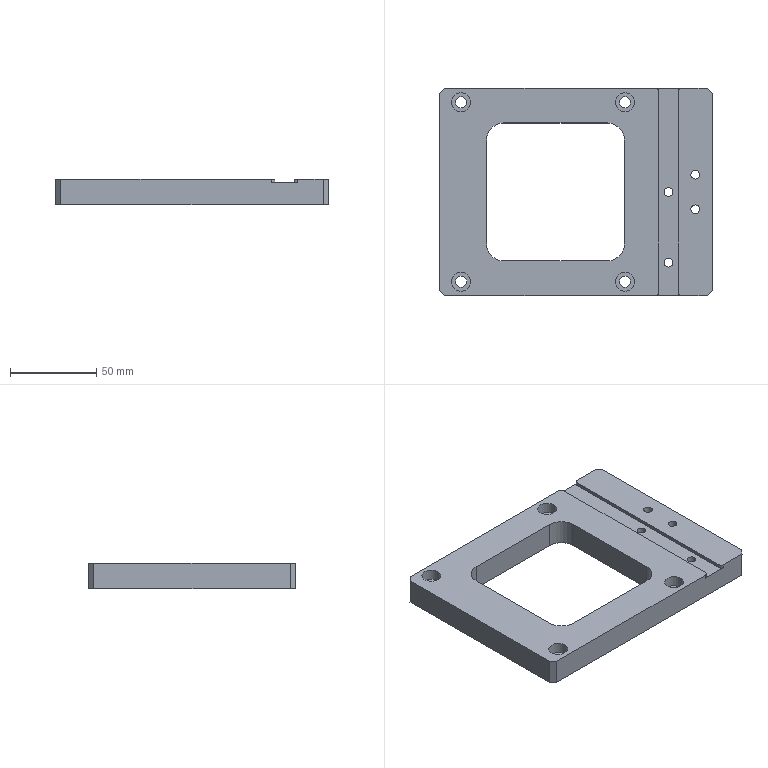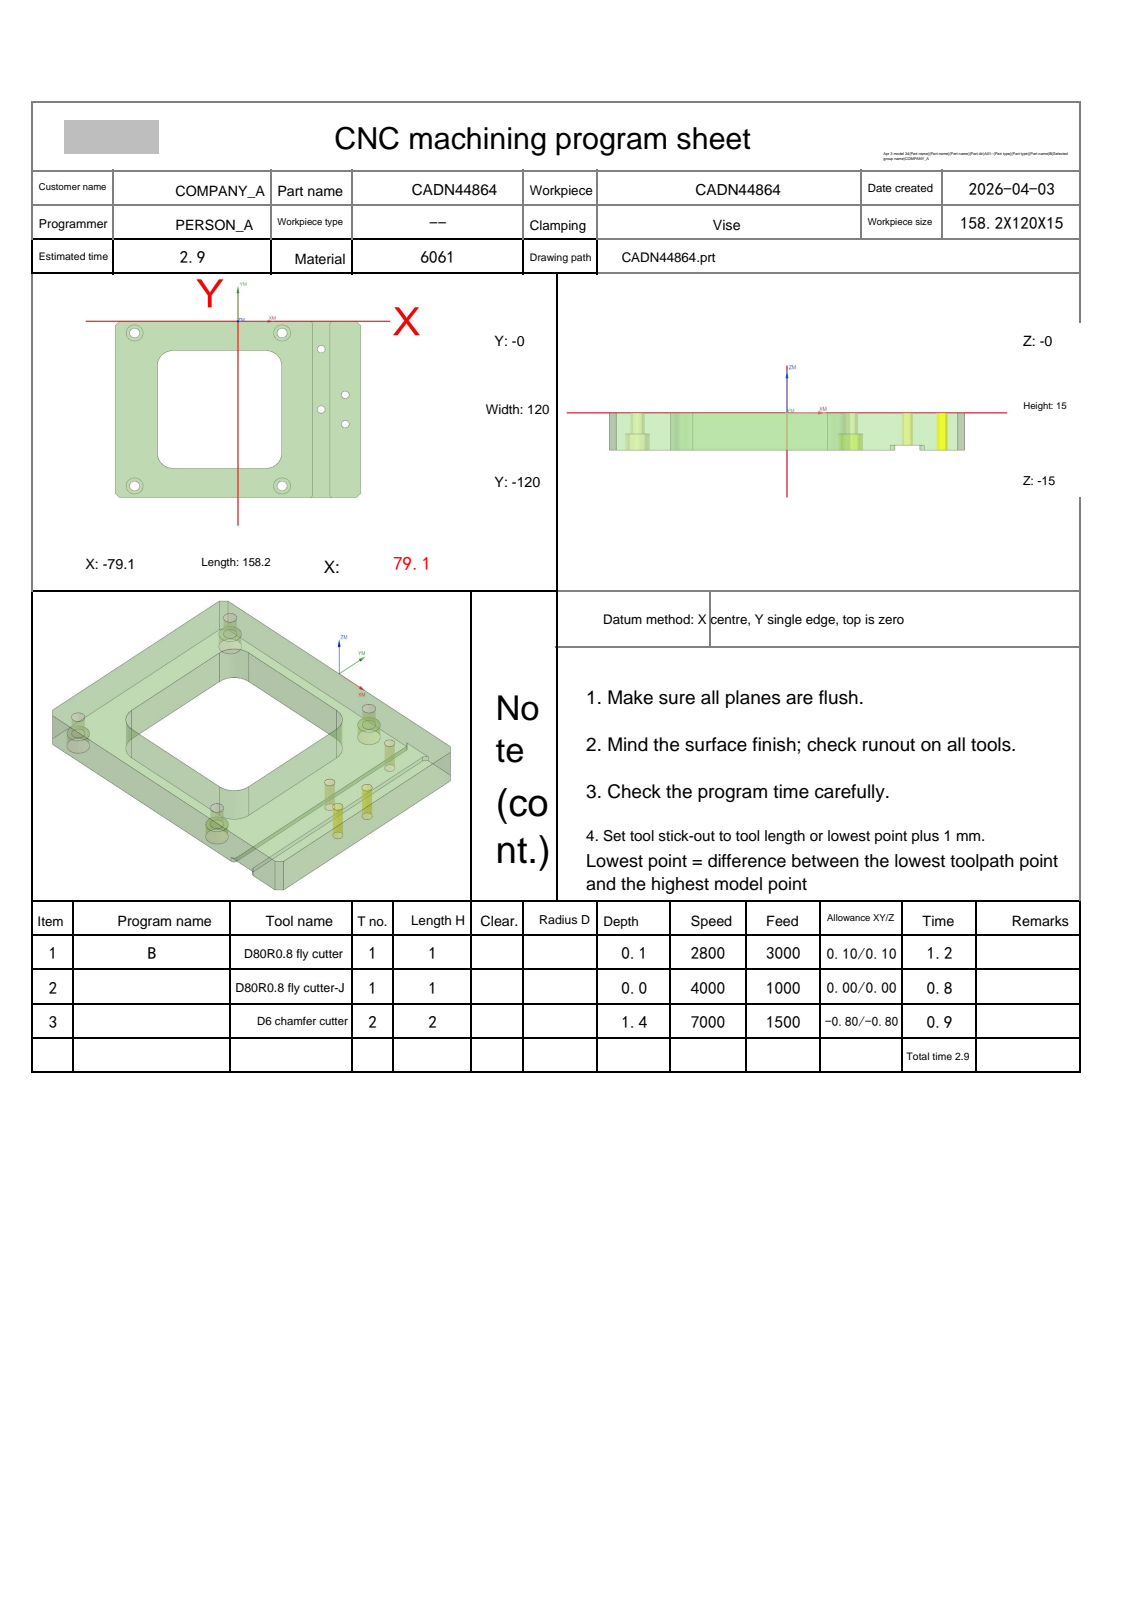NC program | NX | posted by the shop | part box 158.2 x 120 x 15 mm
Whole program:
%
O0001
(Machine time: 3.49 MIN)
(===Total Tool:2===)
(T1=D80R0.8 fly cutter D=80.  R=0.8  D-  H01 Z=-0.   )
(T2=D6 chamfer cutter   D=6.   R=0.   D-  H02 Z=-1.4  )
G80 G90 G17 G49 G40
G91 G28 Z0
M01
N1 T01 M06
(D80R0.8 fly cutter  D=80. R=0.8 H=01 ce=0.10 di=0.10)
G00 G90 G54 X131.197 Y-96.097 M03 S2800
G43 H01 Z20.
M08
Z4.517
G01 Z2.517 F3000.
X119.197
X-111.2
G02 X-119.197 Y-88.1 I.003 J8.
G01 Y-39.26
G02 X-111.2 Y-31.263 I8. J-.003
G01 X119.197
X131.197
Z4.517
G00 Y-96.097
Z4.033
G01 Z2.033
X119.197
X-111.2
G02 X-119.197 Y-88.1 I.003 J8.
G01 Y-39.26
G02 X-111.2 Y-31.263 I8. J-.003
G01 X119.197
X131.197
Z4.033
G00 Y-96.097
Z3.55
G01 Z1.55
X119.197
X-111.2
G02 X-119.197 Y-88.1 I.003 J8.
G01 Y-39.26
G02 X-111.2 Y-31.263 I8. J-.003
G01 X119.197
X131.197
Z3.55
G00 Y-96.097
Z3.067
G01 Z1.067
X119.197
X-111.2
G02 X-119.197 Y-88.1 I.003 J8.
G01 Y-39.26
G02 X-111.2 Y-31.263 I8. J-.003
G01 X119.197
X131.197
Z3.067
G00 Y-96.097
Z2.583
G01 Z.583
X119.197
X-111.2
G02 X-119.197 Y-88.1 I.003 J8.
G01 Y-39.26
G02 X-111.2 Y-31.263 I8. J-.003
G01 X119.197
X131.197
Z2.583
G00 Y-96.097
Z2.1
G01 Z.1
X119.197
X-111.2
G02 X-119.197 Y-88.1 I.003 J8.
G01 Y-39.26
G02 X-111.2 Y-31.263 I8. J-.003
G01 X119.197
X131.197
Z2.1
G00 Z20.
G91 G28 Z0.0
M05
M09
G91 G28 Z0.0
M01
N2 T01 M06
(D80R0.8 fly cutter-J  D=80. R=0.8 H=01 ce=0.00 di=0.00)
G00 G90 G54 X131.099 Y-95.999 M03 S4000
G43 H01 Z20.
M08
Z2.
G01 Z0.0 F1000.
X119.099
X-111.899
G02 X-119.099 Y-88.799 I0.0 J7.2
G01 Y-71.68
G02 X-111.099 Y-63.68 I8. J0.0
G01 X111.899
G03 X119.099 Y-56.48 I0.0 J7.2
G01 Y-39.361
G03 X111.099 Y-31.361 I-8. J0.0
G01 X-119.099
X-131.099
Z2.
G00 Z20.
G91 G28 Z0.0
M05
M09
G91 G28 Z0.0
M01
N3 T02 M06
(D6 chamfer cutter  D=6. R=0. H=02 ce=-0.80 di=-0.80)
G00 G90 G54 X69.332 Y-70.87 M03 S6000
G43 H02 Z20.
M08
Z-.9
G01 Z-1.4 F600.
X69.5 Y-71.5
G03 X71. Y-70. I0.0 J1.5
X69.1 Y-68.1 I-1.9 J0.0
X67.2 Y-70. I0.0 J-1.9
X69.1 Y-71.9 I1.9 J0.0
X71. Y-70. I0.0 J1.9
X69.5 Y-68.5 I-1.5 J0.0
G01 X69.332 Y-69.13
Z-.9
G00 Z20.
X53.832 Y-60.87
Z-.9
G01 Z-1.4
X54. Y-61.5
G03 X55.5 Y-60. I0.0 J1.5
X53.6 Y-58.1 I-1.9 J0.0
X51.7 Y-60. I0.0 J-1.9
X53.6 Y-61.9 I1.9 J0.0
X55.5 Y-60. I0.0 J1.9
X54. Y-58.5 I-1.5 J0.0
G01 X53.832 Y-59.13
Z-.9
G00 Z20.
X69.332 Y-50.87
Z-.9
G01 Z-1.4
X69.5 Y-51.5
G03 X71. Y-50. I0.0 J1.5
X69.1 Y-48.1 I-1.9 J0.0
X67.2 Y-50. I0.0 J-1.9
X69.1 Y-51.9 I1.9 J0.0
X71. Y-50. I0.0 J1.9
X69.5 Y-48.5 I-1.5 J0.0
G01 X69.332 Y-49.13
Z-.9
G00 Z20.
X53.832 Y-19.87
Z-.9
G01 Z-1.4
X54. Y-20.5
G03 X55.5 Y-19. I0.0 J1.5
X53.6 Y-17.1 I-1.9 J0.0
X51.7 Y-19. I0.0 J-1.9
X53.6 Y-20.9 I1.9 J0.0
X55.5 Y-19. I0.0 J1.9
X54. Y-17.5 I-1.5 J0.0
G01 X53.832 Y-18.13
Z-.9
G00 Z20.
G00 G90 X-66.143 Y-9.055 M03 S6000
Z20.
Z-.9
G01 Z-1.4 F600.
X-65.95 Y-9.5
G03 X-64.45 Y-8. I0.0 J1.5
X-66.6 Y-5.85 I-2.15 J0.0
X-68.75 Y-8. I0.0 J-2.15
X-66.6 Y-10.15 I2.15 J0.0
X-64.45 Y-8. I0.0 J2.15
X-65.95 Y-6.5 I-1.5 J0.0
G01 X-66.143 Y-6.945
Z-.9
G00 Z20.
X28.857 Y-9.055
Z-.9
G01 Z-1.4
X29.05 Y-9.5
G03 X30.55 Y-8. I0.0 J1.5
X28.4 Y-5.85 I-2.15 J0.0
X26.25 Y-8. I0.0 J-2.15
X28.4 Y-10.15 I2.15 J0.0
X30.55 Y-8. I0.0 J2.15
X29.05 Y-6.5 I-1.5 J0.0
G01 X28.857 Y-6.945
Z-.9
G00 Z20.
Y-113.055
Z-.9
G01 Z-1.4
X29.05 Y-113.5
G03 X30.55 Y-112. I0.0 J1.5
X28.4 Y-109.85 I-2.15 J0.0
X26.25 Y-112. I0.0 J-2.15
X28.4 Y-114.15 I2.15 J0.0
X30.55 Y-112. I0.0 J2.15
X29.05 Y-110.5 I-1.5 J0.0
G01 X28.857 Y-110.945
Z-.9
G00 Z20.
X-66.143 Y-113.055
Z-.9
G01 Z-1.4
X-65.95 Y-113.5
G03 X-64.45 Y-112. I0.0 J1.5
X-66.6 Y-109.85 I-2.15 J0.0
X-68.75 Y-112. I0.0 J-2.15
X-66.6 Y-114.15 I2.15 J0.0
X-64.45 Y-112. I0.0 J2.15
X-65.95 Y-110.5 I-1.5 J0.0
G01 X-66.143 Y-110.945
Z-.9
G00 Z20.
G00 G90 X-79.8 Y-11.954 M03 S7000
Z20.
Z2.5
G01 Y-3.047 Z-.742 F1500.
X-79.762 Y-2.84 Z-.819
X-79.681 Y-2.645 Z-.895
X-79.562 Y-2.472 Z-.972
X-79.507 Y-2.417 Z-1.
X-76.683 Y.407
G02 X-75.976 Y.7 I.707 J-.707
G01 X75.976
G02 X76.683 Y.407 I0.0 J-1.
G01 X79.507 Y-2.417
G02 X79.8 Y-3.124 I-.707 J-.707
G01 Y-116.876
G02 X79.507 Y-117.583 I-1. J0.0
G01 X76.683 Y-120.407
G02 X75.976 Y-120.7 I-.707 J.707
G01 X-75.976
G02 X-76.683 Y-120.407 I0.0 J1.
G01 X-79.507 Y-117.583
G02 X-79.8 Y-116.876 I.707 J.707
G01 Y-3.124
G02 X-79.507 Y-2.417 I1. J0.0
G01 X-79.154 Y-2.064
Z1.5
G00 Z20.
X-51.2 Y-80.384
Z2.5
G01 Y-90. Z-1.
G03 X-41.9 Y-99.3 I9.3 J0.0
G01 X18.1
G03 X27.4 Y-90. I0.0 J9.3
G01 Y-30.
G03 X18.1 Y-20.7 I-9.3 J0.0
G01 X-41.9
G03 X-51.2 Y-30. I0.0 J-9.3
G01 Y-90.
G03 X-51.187 Y-90.5 I9.3 J0.0
G01 Z1.5
G00 Z20.
M05
M09
G91 G28 Z0.0
G91 G28 Y0.0
M30
%